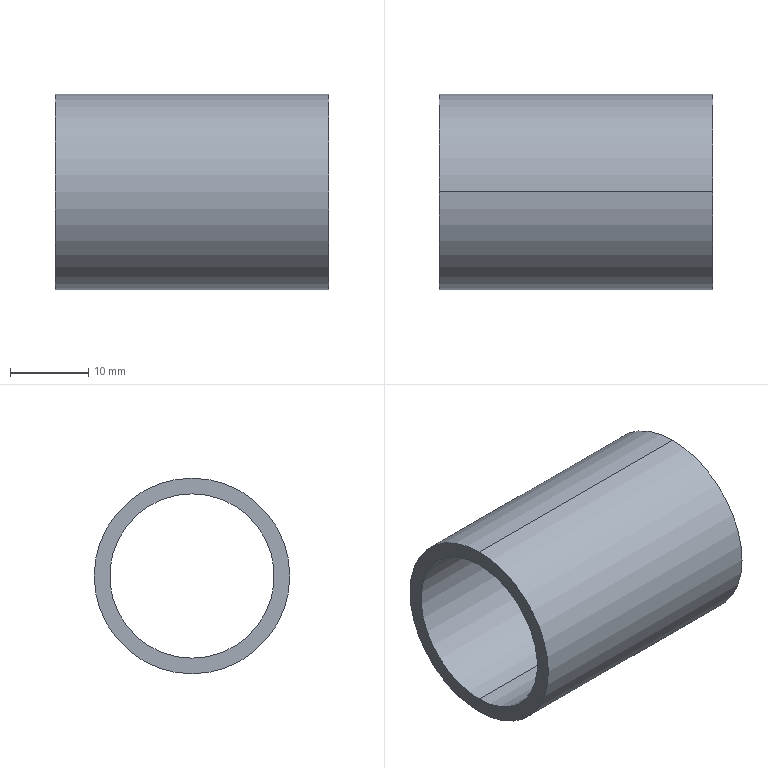Part | SolidWorks | features BaseBody 1 | 1 solid | 6 faces | box 35 x 25 x 25 mm | volume 5058 mm3 | cylinder 4 | plane 2 | commonest cylinder face diameters 21 x2 25 x2
STEP:
#1=CARTESIAN_POINT('',(35.,0.,12.5));
#2=VERTEX_POINT('',#1);
#3=CARTESIAN_POINT('',(35.,0.,-12.5));
#4=VERTEX_POINT('',#3);
#5=CARTESIAN_POINT('',(35.,0.,0.));
#6=DIRECTION('',(-1.,0.,0.));
#7=DIRECTION('',(0.,0.,1.));
#8=AXIS2_PLACEMENT_3D('',#5,#6,#7);
#9=CIRCLE('',#8,12.5);
#10=EDGE_CURVE('',#2,#4,#9,.T.);
#11=ORIENTED_EDGE('',*,*,#10,.T.);
#12=CARTESIAN_POINT('',(0.,0.,-12.5));
#13=VERTEX_POINT('',#12);
#14=CARTESIAN_POINT('',(35.,0.,-12.5));
#15=DIRECTION('',(-1.,0.,0.));
#16=VECTOR('',#15,1000.);
#17=LINE('',#14,#16);
#18=EDGE_CURVE('',#4,#13,#17,.T.);
#19=ORIENTED_EDGE('',*,*,#18,.T.);
#20=CARTESIAN_POINT('',(0.,0.,12.5));
#21=VERTEX_POINT('',#20);
#22=CARTESIAN_POINT('',(0.,0.,0.));
#23=DIRECTION('',(1.,0.,0.));
#24=DIRECTION('',(0.,0.,1.));
#25=AXIS2_PLACEMENT_3D('',#22,#23,#24);
#26=CIRCLE('',#25,12.5);
#27=EDGE_CURVE('',#13,#21,#26,.T.);
#28=ORIENTED_EDGE('',*,*,#27,.T.);
#29=CARTESIAN_POINT('',(35.,0.,12.5));
#30=DIRECTION('',(-1.,0.,0.));
#31=VECTOR('',#30,1000.);
#32=LINE('',#29,#31);
#33=EDGE_CURVE('',#2,#21,#32,.T.);
#34=ORIENTED_EDGE('',*,*,#33,.F.);
#35=EDGE_LOOP('',(#11,#19,#28,#34));
#36=FACE_OUTER_BOUND('',#35,.T.);
#37=CARTESIAN_POINT('',(35.,0.,0.));
#38=DIRECTION('',(-1.,0.,0.));
#39=DIRECTION('',(0.,0.,1.));
#40=AXIS2_PLACEMENT_3D('',#37,#38,#39);
#41=CYLINDRICAL_SURFACE('',#40,12.5);
#42=ADVANCED_FACE('',(#36),#41,.T.);
#43=CARTESIAN_POINT('',(35.,0.,-10.5));
#44=VERTEX_POINT('',#43);
#45=CARTESIAN_POINT('',(35.,0.,10.5));
#46=VERTEX_POINT('',#45);
#47=CARTESIAN_POINT('',(35.,0.,0.));
#48=DIRECTION('',(-1.,0.,0.));
#49=DIRECTION('',(0.,0.,1.));
#50=AXIS2_PLACEMENT_3D('',#47,#48,#49);
#51=CIRCLE('',#50,10.5);
#52=EDGE_CURVE('',#44,#46,#51,.T.);
#53=ORIENTED_EDGE('',*,*,#52,.F.);
#54=CARTESIAN_POINT('',(0.,0.,-10.5));
#55=VERTEX_POINT('',#54);
#56=CARTESIAN_POINT('',(35.,0.,-10.5));
#57=DIRECTION('',(-1.,0.,0.));
#58=VECTOR('',#57,1000.);
#59=LINE('',#56,#58);
#60=EDGE_CURVE('',#44,#55,#59,.T.);
#61=ORIENTED_EDGE('',*,*,#60,.T.);
#62=CARTESIAN_POINT('',(0.,0.,10.5));
#63=VERTEX_POINT('',#62);
#64=CARTESIAN_POINT('',(0.,0.,0.));
#65=DIRECTION('',(-1.,0.,0.));
#66=DIRECTION('',(0.,0.,1.));
#67=AXIS2_PLACEMENT_3D('',#64,#65,#66);
#68=CIRCLE('',#67,10.5);
#69=EDGE_CURVE('',#55,#63,#68,.T.);
#70=ORIENTED_EDGE('',*,*,#69,.T.);
#71=CARTESIAN_POINT('',(35.,0.,10.5));
#72=DIRECTION('',(-1.,0.,0.));
#73=VECTOR('',#72,1000.);
#74=LINE('',#71,#73);
#75=EDGE_CURVE('',#46,#63,#74,.T.);
#76=ORIENTED_EDGE('',*,*,#75,.F.);
#77=EDGE_LOOP('',(#53,#61,#70,#76));
#78=FACE_OUTER_BOUND('',#77,.T.);
#79=CARTESIAN_POINT('',(35.,0.,0.));
#80=DIRECTION('',(-1.,0.,0.));
#81=DIRECTION('',(0.,0.,1.));
#82=AXIS2_PLACEMENT_3D('',#79,#80,#81);
#83=CYLINDRICAL_SURFACE('',#82,10.5);
#84=ADVANCED_FACE('',(#78),#83,.F.);
#85=ORIENTED_EDGE('',*,*,#18,.F.);
#86=CARTESIAN_POINT('',(35.,0.,0.));
#87=DIRECTION('',(-1.,0.,0.));
#88=DIRECTION('',(0.,0.,1.));
#89=AXIS2_PLACEMENT_3D('',#86,#87,#88);
#90=CIRCLE('',#89,12.5);
#91=EDGE_CURVE('',#4,#2,#90,.T.);
#92=ORIENTED_EDGE('',*,*,#91,.T.);
#93=ORIENTED_EDGE('',*,*,#33,.T.);
#94=CARTESIAN_POINT('',(0.,0.,0.));
#95=DIRECTION('',(1.,0.,0.));
#96=DIRECTION('',(0.,0.,1.));
#97=AXIS2_PLACEMENT_3D('',#94,#95,#96);
#98=CIRCLE('',#97,12.5);
#99=EDGE_CURVE('',#21,#13,#98,.T.);
#100=ORIENTED_EDGE('',*,*,#99,.T.);
#101=EDGE_LOOP('',(#85,#92,#93,#100));
#102=FACE_OUTER_BOUND('',#101,.T.);
#103=CARTESIAN_POINT('',(35.,0.,0.));
#104=DIRECTION('',(-1.,0.,0.));
#105=DIRECTION('',(0.,0.,1.));
#106=AXIS2_PLACEMENT_3D('',#103,#104,#105);
#107=CYLINDRICAL_SURFACE('',#106,12.5);
#108=ADVANCED_FACE('',(#102),#107,.T.);
#109=CARTESIAN_POINT('',(0.,0.,0.));
#110=DIRECTION('',(-1.,0.,0.));
#111=DIRECTION('',(0.,0.,1.));
#112=AXIS2_PLACEMENT_3D('',#109,#110,#111);
#113=CIRCLE('',#112,10.5);
#114=EDGE_CURVE('',#63,#55,#113,.T.);
#115=ORIENTED_EDGE('',*,*,#114,.F.);
#116=ORIENTED_EDGE('',*,*,#69,.F.);
#117=EDGE_LOOP('',(#115,#116));
#118=FACE_BOUND('',#117,.T.);
#119=ORIENTED_EDGE('',*,*,#99,.F.);
#120=ORIENTED_EDGE('',*,*,#27,.F.);
#121=EDGE_LOOP('',(#119,#120));
#122=FACE_OUTER_BOUND('',#121,.T.);
#123=CARTESIAN_POINT('',(0.,0.,0.));
#124=DIRECTION('',(1.,0.,0.));
#125=DIRECTION('',(0.,0.,-1.));
#126=AXIS2_PLACEMENT_3D('',#123,#124,#125);
#127=PLANE('',#126);
#128=ADVANCED_FACE('',(#118,#122),#127,.F.);
#129=CARTESIAN_POINT('',(35.,0.,0.));
#130=DIRECTION('',(-1.,0.,0.));
#131=DIRECTION('',(0.,0.,1.));
#132=AXIS2_PLACEMENT_3D('',#129,#130,#131);
#133=CIRCLE('',#132,10.5);
#134=EDGE_CURVE('',#46,#44,#133,.T.);
#135=ORIENTED_EDGE('',*,*,#134,.T.);
#136=ORIENTED_EDGE('',*,*,#52,.T.);
#137=EDGE_LOOP('',(#135,#136));
#138=FACE_BOUND('',#137,.T.);
#139=ORIENTED_EDGE('',*,*,#10,.F.);
#140=ORIENTED_EDGE('',*,*,#91,.F.);
#141=EDGE_LOOP('',(#139,#140));
#142=FACE_OUTER_BOUND('',#141,.T.);
#143=CARTESIAN_POINT('',(35.,0.,0.));
#144=DIRECTION('',(1.,0.,0.));
#145=DIRECTION('',(0.,0.,-1.));
#146=AXIS2_PLACEMENT_3D('',#143,#144,#145);
#147=PLANE('',#146);
#148=ADVANCED_FACE('',(#138,#142),#147,.T.);
#149=ORIENTED_EDGE('',*,*,#60,.F.);
#150=ORIENTED_EDGE('',*,*,#134,.F.);
#151=ORIENTED_EDGE('',*,*,#75,.T.);
#152=ORIENTED_EDGE('',*,*,#114,.T.);
#153=EDGE_LOOP('',(#149,#150,#151,#152));
#154=FACE_OUTER_BOUND('',#153,.T.);
#155=CARTESIAN_POINT('',(35.,0.,0.));
#156=DIRECTION('',(-1.,0.,0.));
#157=DIRECTION('',(0.,0.,1.));
#158=AXIS2_PLACEMENT_3D('',#155,#156,#157);
#159=CYLINDRICAL_SURFACE('',#158,10.5);
#160=ADVANCED_FACE('',(#154),#159,.F.);
#161=CLOSED_SHELL('',(#42,#84,#108,#128,#148,#160));
#162=MANIFOLD_SOLID_BREP('',#161);
#163=CARTESIAN_POINT('',(0.,0.,0.));
#164=DIRECTION('',(0.,0.,1.));
#165=DIRECTION('',(1.,0.,0.));
#166=AXIS2_PLACEMENT_3D('',#163,#164,#165);
#167=(LENGTH_UNIT()NAMED_UNIT(*)SI_UNIT(.MILLI.,.METRE.));
#168=UNCERTAINTY_MEASURE_WITH_UNIT(LENGTH_MEASURE(0.00001),#167,'','');
#169=(NAMED_UNIT(*)PLANE_ANGLE_UNIT()SI_UNIT($,.RADIAN.));
#170=(NAMED_UNIT(*)SI_UNIT($,.STERADIAN.)SOLID_ANGLE_UNIT());
#171=(GEOMETRIC_REPRESENTATION_CONTEXT(3)GLOBAL_UNCERTAINTY_ASSIGNED_CONTEXT((#168))GLOBAL_UNIT_ASSIGNED_CONTEXT((#167,#169,#170))REPRESENTATION_CONTEXT('',''));
#172=ADVANCED_BREP_SHAPE_REPRESENTATION('',(#162,#166),#171);